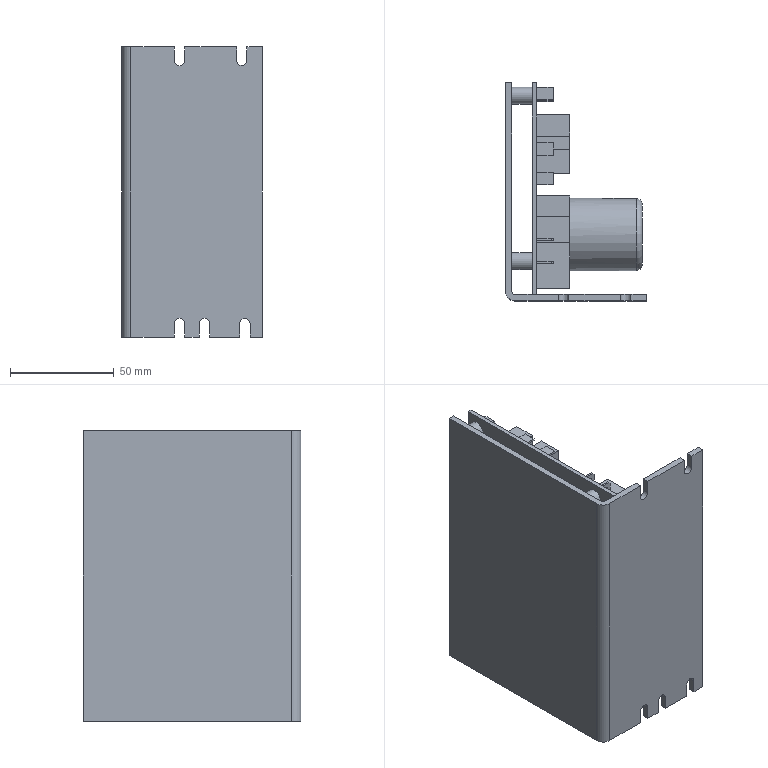Part | STEP file | RUNMCI-615 | 1 solid | 163 faces | box 68 x 105 x 140 mm | volume 172044 mm3 | plane 146 | cylinder 16 | torus 1 | commonest cylinder face diameters 5 x5 2 x4 8 x4 3 x1 9 x1 35 x1